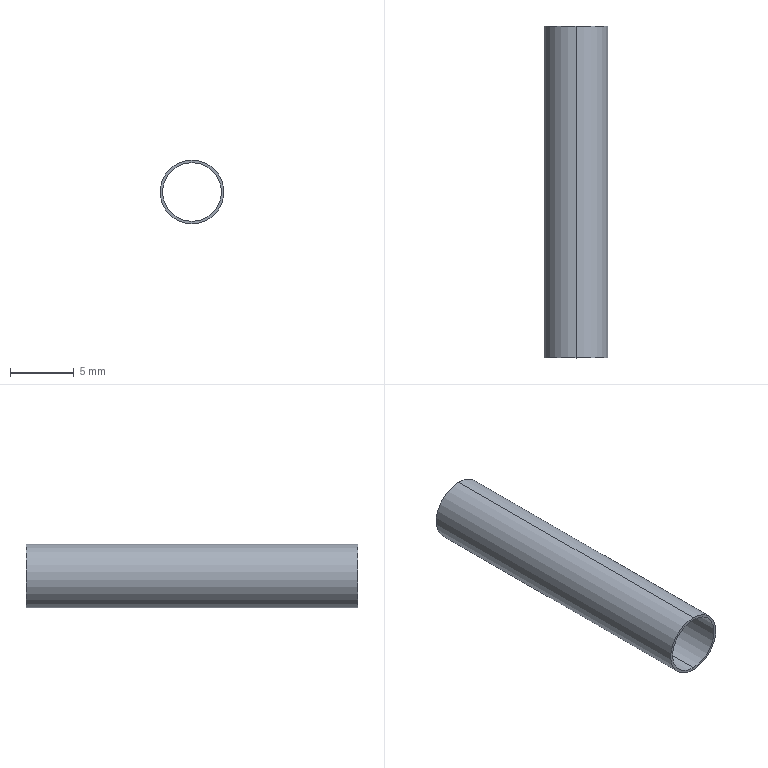Part | SolidWorks | features Extrusion 1 | 1 solid | 6 faces | box 5 x 26 x 5 mm | volume 78.414 mm3 | cylinder 4 | plane 2 | commonest cylinder face diameters 4.6 x2 5 x2
STEP:
#1=CARTESIAN_POINT('',(0.,26.,-2.3));
#2=VERTEX_POINT('',#1);
#3=CARTESIAN_POINT('',(0.,26.,2.3));
#4=VERTEX_POINT('',#3);
#5=CARTESIAN_POINT('',(0.,26.,0.));
#6=DIRECTION('',(0.,1.,0.));
#7=DIRECTION('',(0.,0.,1.));
#8=AXIS2_PLACEMENT_3D('',#5,#6,#7);
#9=CIRCLE('',#8,2.3);
#10=EDGE_CURVE('',#2,#4,#9,.T.);
#11=ORIENTED_EDGE('',*,*,#10,.T.);
#12=CARTESIAN_POINT('',(0.,0.,2.3));
#13=VERTEX_POINT('',#12);
#14=CARTESIAN_POINT('',(0.,26.,2.3));
#15=DIRECTION('',(0.,-1.,0.));
#16=VECTOR('',#15,1000.);
#17=LINE('',#14,#16);
#18=EDGE_CURVE('',#4,#13,#17,.T.);
#19=ORIENTED_EDGE('',*,*,#18,.T.);
#20=CARTESIAN_POINT('',(0.,0.,-2.3));
#21=VERTEX_POINT('',#20);
#22=CARTESIAN_POINT('',(0.,0.,0.));
#23=DIRECTION('',(0.,1.,0.));
#24=DIRECTION('',(0.,0.,1.));
#25=AXIS2_PLACEMENT_3D('',#22,#23,#24);
#26=CIRCLE('',#25,2.3);
#27=EDGE_CURVE('',#21,#13,#26,.T.);
#28=ORIENTED_EDGE('',*,*,#27,.F.);
#29=CARTESIAN_POINT('',(0.,26.,-2.3));
#30=DIRECTION('',(0.,-1.,0.));
#31=VECTOR('',#30,1000.);
#32=LINE('',#29,#31);
#33=EDGE_CURVE('',#2,#21,#32,.T.);
#34=ORIENTED_EDGE('',*,*,#33,.F.);
#35=EDGE_LOOP('',(#11,#19,#28,#34));
#36=FACE_OUTER_BOUND('',#35,.T.);
#37=CARTESIAN_POINT('',(0.,26.,0.));
#38=DIRECTION('',(0.,-1.,0.));
#39=DIRECTION('',(0.,0.,-1.));
#40=AXIS2_PLACEMENT_3D('',#37,#38,#39);
#41=CYLINDRICAL_SURFACE('',#40,2.3);
#42=ADVANCED_FACE('',(#36),#41,.F.);
#43=CARTESIAN_POINT('',(0.,26.,2.5));
#44=VERTEX_POINT('',#43);
#45=CARTESIAN_POINT('',(0.,26.,-2.5));
#46=VERTEX_POINT('',#45);
#47=CARTESIAN_POINT('',(0.,26.,0.));
#48=DIRECTION('',(0.,1.,0.));
#49=DIRECTION('',(0.,0.,1.));
#50=AXIS2_PLACEMENT_3D('',#47,#48,#49);
#51=CIRCLE('',#50,2.5);
#52=EDGE_CURVE('',#44,#46,#51,.T.);
#53=ORIENTED_EDGE('',*,*,#52,.F.);
#54=CARTESIAN_POINT('',(0.,0.,2.5));
#55=VERTEX_POINT('',#54);
#56=CARTESIAN_POINT('',(0.,26.,2.5));
#57=DIRECTION('',(0.,-1.,0.));
#58=VECTOR('',#57,1000.);
#59=LINE('',#56,#58);
#60=EDGE_CURVE('',#44,#55,#59,.T.);
#61=ORIENTED_EDGE('',*,*,#60,.T.);
#62=CARTESIAN_POINT('',(0.,0.,-2.5));
#63=VERTEX_POINT('',#62);
#64=CARTESIAN_POINT('',(0.,0.,0.));
#65=DIRECTION('',(0.,1.,0.));
#66=DIRECTION('',(0.,0.,1.));
#67=AXIS2_PLACEMENT_3D('',#64,#65,#66);
#68=CIRCLE('',#67,2.5);
#69=EDGE_CURVE('',#55,#63,#68,.T.);
#70=ORIENTED_EDGE('',*,*,#69,.T.);
#71=CARTESIAN_POINT('',(0.,26.,-2.5));
#72=DIRECTION('',(0.,-1.,0.));
#73=VECTOR('',#72,1000.);
#74=LINE('',#71,#73);
#75=EDGE_CURVE('',#46,#63,#74,.T.);
#76=ORIENTED_EDGE('',*,*,#75,.F.);
#77=EDGE_LOOP('',(#53,#61,#70,#76));
#78=FACE_OUTER_BOUND('',#77,.T.);
#79=CARTESIAN_POINT('',(0.,26.,0.));
#80=DIRECTION('',(0.,-1.,0.));
#81=DIRECTION('',(0.,0.,-1.));
#82=AXIS2_PLACEMENT_3D('',#79,#80,#81);
#83=CYLINDRICAL_SURFACE('',#82,2.5);
#84=ADVANCED_FACE('',(#78),#83,.T.);
#85=CARTESIAN_POINT('',(0.,26.,0.));
#86=DIRECTION('',(0.,1.,0.));
#87=DIRECTION('',(0.,0.,1.));
#88=AXIS2_PLACEMENT_3D('',#85,#86,#87);
#89=CIRCLE('',#88,2.5);
#90=EDGE_CURVE('',#46,#44,#89,.T.);
#91=ORIENTED_EDGE('',*,*,#90,.T.);
#92=ORIENTED_EDGE('',*,*,#52,.T.);
#93=EDGE_LOOP('',(#91,#92));
#94=FACE_OUTER_BOUND('',#93,.T.);
#95=ORIENTED_EDGE('',*,*,#10,.F.);
#96=CARTESIAN_POINT('',(0.,26.,0.));
#97=DIRECTION('',(0.,1.,0.));
#98=DIRECTION('',(0.,0.,1.));
#99=AXIS2_PLACEMENT_3D('',#96,#97,#98);
#100=CIRCLE('',#99,2.3);
#101=EDGE_CURVE('',#4,#2,#100,.T.);
#102=ORIENTED_EDGE('',*,*,#101,.F.);
#103=EDGE_LOOP('',(#95,#102));
#104=FACE_BOUND('',#103,.T.);
#105=CARTESIAN_POINT('',(0.,26.,0.));
#106=DIRECTION('',(0.,1.,0.));
#107=DIRECTION('',(0.,0.,1.));
#108=AXIS2_PLACEMENT_3D('',#105,#106,#107);
#109=PLANE('',#108);
#110=ADVANCED_FACE('',(#94,#104),#109,.T.);
#111=CARTESIAN_POINT('',(0.,0.,0.));
#112=DIRECTION('',(0.,1.,0.));
#113=DIRECTION('',(0.,0.,1.));
#114=AXIS2_PLACEMENT_3D('',#111,#112,#113);
#115=CIRCLE('',#114,2.5);
#116=EDGE_CURVE('',#63,#55,#115,.T.);
#117=ORIENTED_EDGE('',*,*,#116,.F.);
#118=ORIENTED_EDGE('',*,*,#69,.F.);
#119=EDGE_LOOP('',(#117,#118));
#120=FACE_OUTER_BOUND('',#119,.T.);
#121=ORIENTED_EDGE('',*,*,#27,.T.);
#122=CARTESIAN_POINT('',(0.,0.,0.));
#123=DIRECTION('',(0.,1.,0.));
#124=DIRECTION('',(0.,0.,1.));
#125=AXIS2_PLACEMENT_3D('',#122,#123,#124);
#126=CIRCLE('',#125,2.3);
#127=EDGE_CURVE('',#13,#21,#126,.T.);
#128=ORIENTED_EDGE('',*,*,#127,.T.);
#129=EDGE_LOOP('',(#121,#128));
#130=FACE_BOUND('',#129,.T.);
#131=CARTESIAN_POINT('',(0.,0.,0.));
#132=DIRECTION('',(0.,1.,0.));
#133=DIRECTION('',(0.,0.,1.));
#134=AXIS2_PLACEMENT_3D('',#131,#132,#133);
#135=PLANE('',#134);
#136=ADVANCED_FACE('',(#120,#130),#135,.F.);
#137=ORIENTED_EDGE('',*,*,#60,.F.);
#138=ORIENTED_EDGE('',*,*,#90,.F.);
#139=ORIENTED_EDGE('',*,*,#75,.T.);
#140=ORIENTED_EDGE('',*,*,#116,.T.);
#141=EDGE_LOOP('',(#137,#138,#139,#140));
#142=FACE_OUTER_BOUND('',#141,.T.);
#143=CARTESIAN_POINT('',(0.,26.,0.));
#144=DIRECTION('',(0.,-1.,0.));
#145=DIRECTION('',(0.,0.,-1.));
#146=AXIS2_PLACEMENT_3D('',#143,#144,#145);
#147=CYLINDRICAL_SURFACE('',#146,2.5);
#148=ADVANCED_FACE('',(#142),#147,.T.);
#149=ORIENTED_EDGE('',*,*,#18,.F.);
#150=ORIENTED_EDGE('',*,*,#101,.T.);
#151=ORIENTED_EDGE('',*,*,#33,.T.);
#152=ORIENTED_EDGE('',*,*,#127,.F.);
#153=EDGE_LOOP('',(#149,#150,#151,#152));
#154=FACE_OUTER_BOUND('',#153,.T.);
#155=CARTESIAN_POINT('',(0.,26.,0.));
#156=DIRECTION('',(0.,-1.,0.));
#157=DIRECTION('',(0.,0.,-1.));
#158=AXIS2_PLACEMENT_3D('',#155,#156,#157);
#159=CYLINDRICAL_SURFACE('',#158,2.3);
#160=ADVANCED_FACE('',(#154),#159,.F.);
#161=CLOSED_SHELL('',(#42,#84,#110,#136,#148,#160));
#162=MANIFOLD_SOLID_BREP('',#161);
#163=CARTESIAN_POINT('',(0.,0.,0.));
#164=DIRECTION('',(0.,0.,1.));
#165=DIRECTION('',(1.,0.,0.));
#166=AXIS2_PLACEMENT_3D('',#163,#164,#165);
#167=(LENGTH_UNIT()NAMED_UNIT(*)SI_UNIT(.MILLI.,.METRE.));
#168=UNCERTAINTY_MEASURE_WITH_UNIT(LENGTH_MEASURE(0.00001),#167,'','');
#169=(NAMED_UNIT(*)PLANE_ANGLE_UNIT()SI_UNIT($,.RADIAN.));
#170=(NAMED_UNIT(*)SI_UNIT($,.STERADIAN.)SOLID_ANGLE_UNIT());
#171=(GEOMETRIC_REPRESENTATION_CONTEXT(3)GLOBAL_UNCERTAINTY_ASSIGNED_CONTEXT((#168))GLOBAL_UNIT_ASSIGNED_CONTEXT((#167,#169,#170))REPRESENTATION_CONTEXT('',''));
#172=ADVANCED_BREP_SHAPE_REPRESENTATION('',(#162,#166),#171);